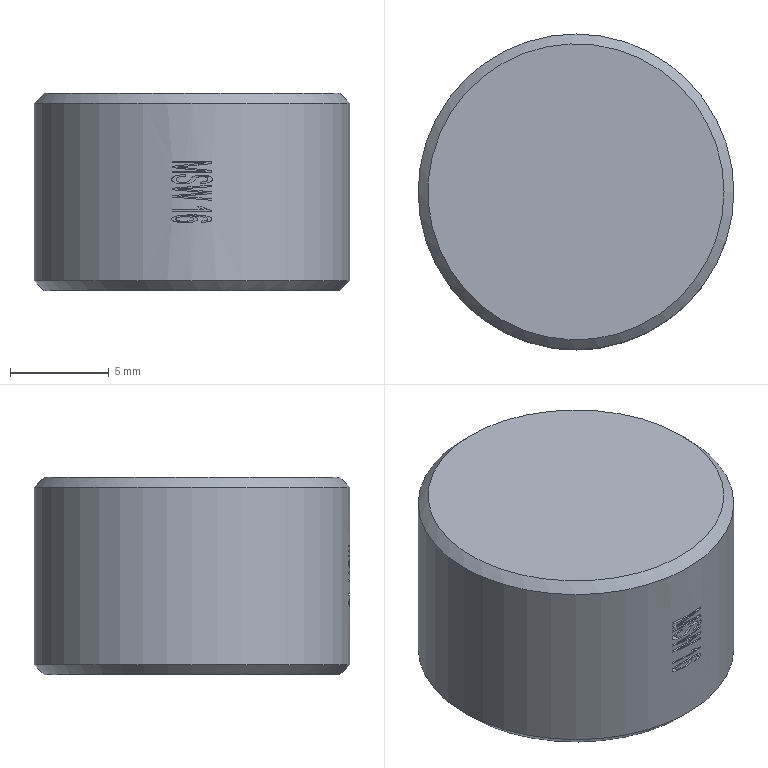Part | STEP file | SWM_id746_x_t | 1 solid | 64 faces | box 16 x 16 x 10 mm | volume 1720 mm3 | plane 40 | other 20 | cylinder 2 | cone 2 | commonest cylinder face diameters 16 x2